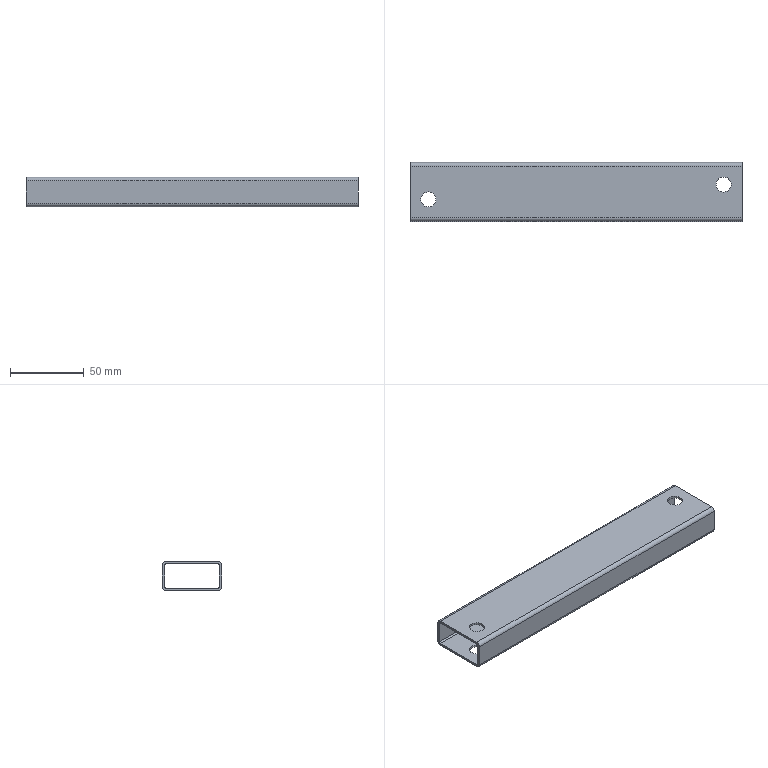Part | STEP file | 6150402 | 1 solid | 22 faces | box 225 x 40 x 20 mm | volume 36971 mm3 | cylinder 12 | plane 10 | commonest cylinder face diameters 2 x4 5 x4 10.2 x4
STEP:
#1=CARTESIAN_POINT('',(225.,17.5,-10.));
#2=VERTEX_POINT('',#1);
#3=CARTESIAN_POINT('',(225.,20.,-7.5));
#4=VERTEX_POINT('',#3);
#5=CARTESIAN_POINT('',(225.,17.5,-7.5));
#6=DIRECTION('',(1.,0.,0.));
#7=DIRECTION('',(0.,0.,-1.));
#8=AXIS2_PLACEMENT_3D('',#5,#6,#7);
#9=CIRCLE('',#8,2.5);
#10=EDGE_CURVE('',#2,#4,#9,.T.);
#11=ORIENTED_EDGE('',*,*,#10,.T.);
#12=CARTESIAN_POINT('',(225.,20.,7.5));
#13=VERTEX_POINT('',#12);
#14=CARTESIAN_POINT('',(225.,20.,7.5));
#15=DIRECTION('',(0.,0.,1.));
#16=VECTOR('',#15,1000.);
#17=LINE('',#14,#16);
#18=EDGE_CURVE('',#4,#13,#17,.T.);
#19=ORIENTED_EDGE('',*,*,#18,.T.);
#20=CARTESIAN_POINT('',(225.,17.5,10.));
#21=VERTEX_POINT('',#20);
#22=CARTESIAN_POINT('',(225.,17.5,7.5));
#23=DIRECTION('',(1.,0.,0.));
#24=DIRECTION('',(0.,0.,-1.));
#25=AXIS2_PLACEMENT_3D('',#22,#23,#24);
#26=CIRCLE('',#25,2.5);
#27=EDGE_CURVE('',#13,#21,#26,.T.);
#28=ORIENTED_EDGE('',*,*,#27,.T.);
#29=CARTESIAN_POINT('',(225.,-17.5,10.));
#30=VERTEX_POINT('',#29);
#31=CARTESIAN_POINT('',(225.,17.5,10.));
#32=DIRECTION('',(0.,-1.,0.));
#33=VECTOR('',#32,1000.);
#34=LINE('',#31,#33);
#35=EDGE_CURVE('',#21,#30,#34,.T.);
#36=ORIENTED_EDGE('',*,*,#35,.T.);
#37=CARTESIAN_POINT('',(225.,-20.,7.5));
#38=VERTEX_POINT('',#37);
#39=CARTESIAN_POINT('',(225.,-17.5,7.5));
#40=DIRECTION('',(1.,0.,0.));
#41=DIRECTION('',(0.,0.,-1.));
#42=AXIS2_PLACEMENT_3D('',#39,#40,#41);
#43=CIRCLE('',#42,2.5);
#44=EDGE_CURVE('',#30,#38,#43,.T.);
#45=ORIENTED_EDGE('',*,*,#44,.T.);
#46=CARTESIAN_POINT('',(225.,-20.,-7.5));
#47=VERTEX_POINT('',#46);
#48=CARTESIAN_POINT('',(225.,-20.,7.5));
#49=DIRECTION('',(0.,0.,-1.));
#50=VECTOR('',#49,1000.);
#51=LINE('',#48,#50);
#52=EDGE_CURVE('',#38,#47,#51,.T.);
#53=ORIENTED_EDGE('',*,*,#52,.T.);
#54=CARTESIAN_POINT('',(225.,-17.5,-10.));
#55=VERTEX_POINT('',#54);
#56=CARTESIAN_POINT('',(225.,-17.5,-7.5));
#57=DIRECTION('',(1.,0.,0.));
#58=DIRECTION('',(0.,0.,1.));
#59=AXIS2_PLACEMENT_3D('',#56,#57,#58);
#60=CIRCLE('',#59,2.5);
#61=EDGE_CURVE('',#47,#55,#60,.T.);
#62=ORIENTED_EDGE('',*,*,#61,.T.);
#63=CARTESIAN_POINT('',(225.,17.5,-10.));
#64=DIRECTION('',(0.,1.,0.));
#65=VECTOR('',#64,1000.);
#66=LINE('',#63,#65);
#67=EDGE_CURVE('',#55,#2,#66,.T.);
#68=ORIENTED_EDGE('',*,*,#67,.T.);
#69=EDGE_LOOP('',(#11,#19,#28,#36,#45,#53,#62,#68));
#70=FACE_OUTER_BOUND('',#69,.T.);
#71=CARTESIAN_POINT('',(225.,17.5,8.5));
#72=VERTEX_POINT('',#71);
#73=CARTESIAN_POINT('',(225.,-17.5,8.5));
#74=VERTEX_POINT('',#73);
#75=CARTESIAN_POINT('',(225.,17.5,8.5));
#76=DIRECTION('',(0.,-1.,0.));
#77=VECTOR('',#76,1000.);
#78=LINE('',#75,#77);
#79=EDGE_CURVE('',#72,#74,#78,.T.);
#80=ORIENTED_EDGE('',*,*,#79,.F.);
#81=CARTESIAN_POINT('',(225.,18.5,7.5));
#82=VERTEX_POINT('',#81);
#83=CARTESIAN_POINT('',(225.,17.5,7.5));
#84=DIRECTION('',(1.,0.,0.));
#85=DIRECTION('',(0.,0.,-1.));
#86=AXIS2_PLACEMENT_3D('',#83,#84,#85);
#87=CIRCLE('',#86,1.);
#88=EDGE_CURVE('',#82,#72,#87,.T.);
#89=ORIENTED_EDGE('',*,*,#88,.F.);
#90=CARTESIAN_POINT('',(225.,18.5,-7.5));
#91=VERTEX_POINT('',#90);
#92=CARTESIAN_POINT('',(225.,18.5,7.5));
#93=DIRECTION('',(0.,0.,1.));
#94=VECTOR('',#93,1000.);
#95=LINE('',#92,#94);
#96=EDGE_CURVE('',#91,#82,#95,.T.);
#97=ORIENTED_EDGE('',*,*,#96,.F.);
#98=CARTESIAN_POINT('',(225.,17.5,-8.5));
#99=VERTEX_POINT('',#98);
#100=CARTESIAN_POINT('',(225.,17.5,-7.5));
#101=DIRECTION('',(1.,0.,0.));
#102=DIRECTION('',(0.,0.,-1.));
#103=AXIS2_PLACEMENT_3D('',#100,#101,#102);
#104=CIRCLE('',#103,1.);
#105=EDGE_CURVE('',#99,#91,#104,.T.);
#106=ORIENTED_EDGE('',*,*,#105,.F.);
#107=CARTESIAN_POINT('',(225.,-17.5,-8.5));
#108=VERTEX_POINT('',#107);
#109=CARTESIAN_POINT('',(225.,17.5,-8.5));
#110=DIRECTION('',(0.,1.,0.));
#111=VECTOR('',#110,1000.);
#112=LINE('',#109,#111);
#113=EDGE_CURVE('',#108,#99,#112,.T.);
#114=ORIENTED_EDGE('',*,*,#113,.F.);
#115=CARTESIAN_POINT('',(225.,-18.5,-7.5));
#116=VERTEX_POINT('',#115);
#117=CARTESIAN_POINT('',(225.,-17.5,-7.5));
#118=DIRECTION('',(1.,0.,0.));
#119=DIRECTION('',(0.,0.,1.));
#120=AXIS2_PLACEMENT_3D('',#117,#118,#119);
#121=CIRCLE('',#120,1.);
#122=EDGE_CURVE('',#116,#108,#121,.T.);
#123=ORIENTED_EDGE('',*,*,#122,.F.);
#124=CARTESIAN_POINT('',(225.,-18.5,7.5));
#125=VERTEX_POINT('',#124);
#126=CARTESIAN_POINT('',(225.,-18.5,7.5));
#127=DIRECTION('',(0.,0.,-1.));
#128=VECTOR('',#127,1000.);
#129=LINE('',#126,#128);
#130=EDGE_CURVE('',#125,#116,#129,.T.);
#131=ORIENTED_EDGE('',*,*,#130,.F.);
#132=CARTESIAN_POINT('',(225.,-17.5,7.5));
#133=DIRECTION('',(1.,0.,0.));
#134=DIRECTION('',(0.,0.,-1.));
#135=AXIS2_PLACEMENT_3D('',#132,#133,#134);
#136=CIRCLE('',#135,1.);
#137=EDGE_CURVE('',#74,#125,#136,.T.);
#138=ORIENTED_EDGE('',*,*,#137,.F.);
#139=EDGE_LOOP('',(#80,#89,#97,#106,#114,#123,#131,#138));
#140=FACE_BOUND('',#139,.T.);
#141=CARTESIAN_POINT('',(225.,17.5,-7.5));
#142=DIRECTION('',(1.,0.,0.));
#143=DIRECTION('',(0.,0.,-1.));
#144=AXIS2_PLACEMENT_3D('',#141,#142,#143);
#145=PLANE('',#144);
#146=ADVANCED_FACE('',(#70,#140),#145,.T.);
#147=CARTESIAN_POINT('',(0.,17.5,-10.));
#148=VERTEX_POINT('',#147);
#149=CARTESIAN_POINT('',(0.,20.,-7.5));
#150=VERTEX_POINT('',#149);
#151=CARTESIAN_POINT('',(0.,17.5,-7.5));
#152=DIRECTION('',(1.,0.,0.));
#153=DIRECTION('',(0.,0.,-1.));
#154=AXIS2_PLACEMENT_3D('',#151,#152,#153);
#155=CIRCLE('',#154,2.5);
#156=EDGE_CURVE('',#148,#150,#155,.T.);
#157=ORIENTED_EDGE('',*,*,#156,.F.);
#158=CARTESIAN_POINT('',(0.,-17.5,-10.));
#159=VERTEX_POINT('',#158);
#160=CARTESIAN_POINT('',(0.,17.5,-10.));
#161=DIRECTION('',(0.,1.,0.));
#162=VECTOR('',#161,1000.);
#163=LINE('',#160,#162);
#164=EDGE_CURVE('',#159,#148,#163,.T.);
#165=ORIENTED_EDGE('',*,*,#164,.F.);
#166=CARTESIAN_POINT('',(0.,-20.,-7.5));
#167=VERTEX_POINT('',#166);
#168=CARTESIAN_POINT('',(0.,-17.5,-7.5));
#169=DIRECTION('',(1.,0.,0.));
#170=DIRECTION('',(0.,0.,1.));
#171=AXIS2_PLACEMENT_3D('',#168,#169,#170);
#172=CIRCLE('',#171,2.5);
#173=EDGE_CURVE('',#167,#159,#172,.T.);
#174=ORIENTED_EDGE('',*,*,#173,.F.);
#175=CARTESIAN_POINT('',(0.,-20.,7.5));
#176=VERTEX_POINT('',#175);
#177=CARTESIAN_POINT('',(0.,-20.,7.5));
#178=DIRECTION('',(0.,0.,-1.));
#179=VECTOR('',#178,1000.);
#180=LINE('',#177,#179);
#181=EDGE_CURVE('',#176,#167,#180,.T.);
#182=ORIENTED_EDGE('',*,*,#181,.F.);
#183=CARTESIAN_POINT('',(0.,-17.5,10.));
#184=VERTEX_POINT('',#183);
#185=CARTESIAN_POINT('',(0.,-17.5,7.5));
#186=DIRECTION('',(1.,0.,0.));
#187=DIRECTION('',(0.,0.,-1.));
#188=AXIS2_PLACEMENT_3D('',#185,#186,#187);
#189=CIRCLE('',#188,2.5);
#190=EDGE_CURVE('',#184,#176,#189,.T.);
#191=ORIENTED_EDGE('',*,*,#190,.F.);
#192=CARTESIAN_POINT('',(0.,17.5,10.));
#193=VERTEX_POINT('',#192);
#194=CARTESIAN_POINT('',(0.,17.5,10.));
#195=DIRECTION('',(0.,-1.,0.));
#196=VECTOR('',#195,1000.);
#197=LINE('',#194,#196);
#198=EDGE_CURVE('',#193,#184,#197,.T.);
#199=ORIENTED_EDGE('',*,*,#198,.F.);
#200=CARTESIAN_POINT('',(0.,20.,7.5));
#201=VERTEX_POINT('',#200);
#202=CARTESIAN_POINT('',(0.,17.5,7.5));
#203=DIRECTION('',(1.,0.,0.));
#204=DIRECTION('',(0.,0.,-1.));
#205=AXIS2_PLACEMENT_3D('',#202,#203,#204);
#206=CIRCLE('',#205,2.5);
#207=EDGE_CURVE('',#201,#193,#206,.T.);
#208=ORIENTED_EDGE('',*,*,#207,.F.);
#209=CARTESIAN_POINT('',(0.,20.,7.5));
#210=DIRECTION('',(0.,0.,1.));
#211=VECTOR('',#210,1000.);
#212=LINE('',#209,#211);
#213=EDGE_CURVE('',#150,#201,#212,.T.);
#214=ORIENTED_EDGE('',*,*,#213,.F.);
#215=EDGE_LOOP('',(#157,#165,#174,#182,#191,#199,#208,#214));
#216=FACE_OUTER_BOUND('',#215,.T.);
#217=CARTESIAN_POINT('',(0.,18.5,7.5));
#218=VERTEX_POINT('',#217);
#219=CARTESIAN_POINT('',(0.,17.5,8.5));
#220=VERTEX_POINT('',#219);
#221=CARTESIAN_POINT('',(0.,17.5,7.5));
#222=DIRECTION('',(1.,0.,0.));
#223=DIRECTION('',(0.,0.,-1.));
#224=AXIS2_PLACEMENT_3D('',#221,#222,#223);
#225=CIRCLE('',#224,1.);
#226=EDGE_CURVE('',#218,#220,#225,.T.);
#227=ORIENTED_EDGE('',*,*,#226,.T.);
#228=CARTESIAN_POINT('',(0.,-17.5,8.5));
#229=VERTEX_POINT('',#228);
#230=CARTESIAN_POINT('',(0.,17.5,8.5));
#231=DIRECTION('',(0.,-1.,0.));
#232=VECTOR('',#231,1000.);
#233=LINE('',#230,#232);
#234=EDGE_CURVE('',#220,#229,#233,.T.);
#235=ORIENTED_EDGE('',*,*,#234,.T.);
#236=CARTESIAN_POINT('',(0.,-18.5,7.5));
#237=VERTEX_POINT('',#236);
#238=CARTESIAN_POINT('',(0.,-17.5,7.5));
#239=DIRECTION('',(1.,0.,0.));
#240=DIRECTION('',(0.,0.,-1.));
#241=AXIS2_PLACEMENT_3D('',#238,#239,#240);
#242=CIRCLE('',#241,1.);
#243=EDGE_CURVE('',#229,#237,#242,.T.);
#244=ORIENTED_EDGE('',*,*,#243,.T.);
#245=CARTESIAN_POINT('',(0.,-18.5,-7.5));
#246=VERTEX_POINT('',#245);
#247=CARTESIAN_POINT('',(0.,-18.5,7.5));
#248=DIRECTION('',(0.,0.,-1.));
#249=VECTOR('',#248,1000.);
#250=LINE('',#247,#249);
#251=EDGE_CURVE('',#237,#246,#250,.T.);
#252=ORIENTED_EDGE('',*,*,#251,.T.);
#253=CARTESIAN_POINT('',(0.,-17.5,-8.5));
#254=VERTEX_POINT('',#253);
#255=CARTESIAN_POINT('',(0.,-17.5,-7.5));
#256=DIRECTION('',(1.,0.,0.));
#257=DIRECTION('',(0.,0.,1.));
#258=AXIS2_PLACEMENT_3D('',#255,#256,#257);
#259=CIRCLE('',#258,1.);
#260=EDGE_CURVE('',#246,#254,#259,.T.);
#261=ORIENTED_EDGE('',*,*,#260,.T.);
#262=CARTESIAN_POINT('',(0.,17.5,-8.5));
#263=VERTEX_POINT('',#262);
#264=CARTESIAN_POINT('',(0.,17.5,-8.5));
#265=DIRECTION('',(0.,1.,0.));
#266=VECTOR('',#265,1000.);
#267=LINE('',#264,#266);
#268=EDGE_CURVE('',#254,#263,#267,.T.);
#269=ORIENTED_EDGE('',*,*,#268,.T.);
#270=CARTESIAN_POINT('',(0.,18.5,-7.5));
#271=VERTEX_POINT('',#270);
#272=CARTESIAN_POINT('',(0.,17.5,-7.5));
#273=DIRECTION('',(1.,0.,0.));
#274=DIRECTION('',(0.,0.,-1.));
#275=AXIS2_PLACEMENT_3D('',#272,#273,#274);
#276=CIRCLE('',#275,1.);
#277=EDGE_CURVE('',#263,#271,#276,.T.);
#278=ORIENTED_EDGE('',*,*,#277,.T.);
#279=CARTESIAN_POINT('',(0.,18.5,7.5));
#280=DIRECTION('',(0.,0.,1.));
#281=VECTOR('',#280,1000.);
#282=LINE('',#279,#281);
#283=EDGE_CURVE('',#271,#218,#282,.T.);
#284=ORIENTED_EDGE('',*,*,#283,.T.);
#285=EDGE_LOOP('',(#227,#235,#244,#252,#261,#269,#278,#284));
#286=FACE_BOUND('',#285,.T.);
#287=CARTESIAN_POINT('',(0.,17.5,-7.5));
#288=DIRECTION('',(1.,0.,0.));
#289=DIRECTION('',(0.,0.,-1.));
#290=AXIS2_PLACEMENT_3D('',#287,#288,#289);
#291=PLANE('',#290);
#292=ADVANCED_FACE('',(#216,#286),#291,.F.);
#293=ORIENTED_EDGE('',*,*,#156,.T.);
#294=CARTESIAN_POINT('',(225.,20.,-7.5));
#295=DIRECTION('',(-1.,0.,0.));
#296=VECTOR('',#295,1000.);
#297=LINE('',#294,#296);
#298=EDGE_CURVE('',#4,#150,#297,.T.);
#299=ORIENTED_EDGE('',*,*,#298,.F.);
#300=ORIENTED_EDGE('',*,*,#10,.F.);
#301=CARTESIAN_POINT('',(225.,17.5,-10.));
#302=DIRECTION('',(-1.,0.,0.));
#303=VECTOR('',#302,1000.);
#304=LINE('',#301,#303);
#305=EDGE_CURVE('',#2,#148,#304,.T.);
#306=ORIENTED_EDGE('',*,*,#305,.T.);
#307=EDGE_LOOP('',(#293,#299,#300,#306));
#308=FACE_OUTER_BOUND('',#307,.T.);
#309=CARTESIAN_POINT('',(225.,17.5,-7.5));
#310=DIRECTION('',(-1.,0.,0.));
#311=DIRECTION('',(0.,0.,1.));
#312=AXIS2_PLACEMENT_3D('',#309,#310,#311);
#313=CYLINDRICAL_SURFACE('',#312,2.5);
#314=ADVANCED_FACE('',(#308),#313,.T.);
#315=ORIENTED_EDGE('',*,*,#213,.T.);
#316=CARTESIAN_POINT('',(225.,20.,7.5));
#317=DIRECTION('',(-1.,0.,0.));
#318=VECTOR('',#317,1000.);
#319=LINE('',#316,#318);
#320=EDGE_CURVE('',#13,#201,#319,.T.);
#321=ORIENTED_EDGE('',*,*,#320,.F.);
#322=ORIENTED_EDGE('',*,*,#18,.F.);
#323=ORIENTED_EDGE('',*,*,#298,.T.);
#324=EDGE_LOOP('',(#315,#321,#322,#323));
#325=FACE_OUTER_BOUND('',#324,.T.);
#326=CARTESIAN_POINT('',(225.,20.,7.5));
#327=DIRECTION('',(0.,-1.,0.));
#328=DIRECTION('',(0.,0.,-1.));
#329=AXIS2_PLACEMENT_3D('',#326,#327,#328);
#330=PLANE('',#329);
#331=ADVANCED_FACE('',(#325),#330,.F.);
#332=ORIENTED_EDGE('',*,*,#207,.T.);
#333=CARTESIAN_POINT('',(225.,17.5,10.));
#334=DIRECTION('',(-1.,0.,0.));
#335=VECTOR('',#334,1000.);
#336=LINE('',#333,#335);
#337=EDGE_CURVE('',#21,#193,#336,.T.);
#338=ORIENTED_EDGE('',*,*,#337,.F.);
#339=ORIENTED_EDGE('',*,*,#27,.F.);
#340=ORIENTED_EDGE('',*,*,#320,.T.);
#341=EDGE_LOOP('',(#332,#338,#339,#340));
#342=FACE_OUTER_BOUND('',#341,.T.);
#343=CARTESIAN_POINT('',(225.,17.5,7.5));
#344=DIRECTION('',(-1.,0.,0.));
#345=DIRECTION('',(0.,0.,1.));
#346=AXIS2_PLACEMENT_3D('',#343,#344,#345);
#347=CYLINDRICAL_SURFACE('',#346,2.5);
#348=ADVANCED_FACE('',(#342),#347,.T.);
#349=CARTESIAN_POINT('',(212.5,10.1,10.));
#350=VERTEX_POINT('',#349);
#351=CARTESIAN_POINT('',(212.5,5.,10.));
#352=DIRECTION('',(0.,0.,-1.));
#353=DIRECTION('',(0.,1.,0.));
#354=AXIS2_PLACEMENT_3D('',#351,#352,#353);
#355=CIRCLE('',#354,5.1);
#356=EDGE_CURVE('',#350,#350,#355,.T.);
#357=ORIENTED_EDGE('',*,*,#356,.T.);
#358=EDGE_LOOP('',(#357));
#359=FACE_BOUND('',#358,.T.);
#360=CARTESIAN_POINT('',(12.5,0.1,10.));
#361=VERTEX_POINT('',#360);
#362=CARTESIAN_POINT('',(12.5,-5.,10.));
#363=DIRECTION('',(0.,0.,-1.));
#364=DIRECTION('',(0.,1.,0.));
#365=AXIS2_PLACEMENT_3D('',#362,#363,#364);
#366=CIRCLE('',#365,5.1);
#367=EDGE_CURVE('',#361,#361,#366,.T.);
#368=ORIENTED_EDGE('',*,*,#367,.T.);
#369=EDGE_LOOP('',(#368));
#370=FACE_BOUND('',#369,.T.);
#371=ORIENTED_EDGE('',*,*,#198,.T.);
#372=CARTESIAN_POINT('',(225.,-17.5,10.));
#373=DIRECTION('',(-1.,0.,0.));
#374=VECTOR('',#373,1000.);
#375=LINE('',#372,#374);
#376=EDGE_CURVE('',#30,#184,#375,.T.);
#377=ORIENTED_EDGE('',*,*,#376,.F.);
#378=ORIENTED_EDGE('',*,*,#35,.F.);
#379=ORIENTED_EDGE('',*,*,#337,.T.);
#380=EDGE_LOOP('',(#371,#377,#378,#379));
#381=FACE_OUTER_BOUND('',#380,.T.);
#382=CARTESIAN_POINT('',(225.,17.5,10.));
#383=DIRECTION('',(0.,0.,-1.));
#384=DIRECTION('',(0.,1.,0.));
#385=AXIS2_PLACEMENT_3D('',#382,#383,#384);
#386=PLANE('',#385);
#387=ADVANCED_FACE('',(#359,#370,#381),#386,.F.);
#388=ORIENTED_EDGE('',*,*,#190,.T.);
#389=CARTESIAN_POINT('',(225.,-20.,7.5));
#390=DIRECTION('',(-1.,0.,0.));
#391=VECTOR('',#390,1000.);
#392=LINE('',#389,#391);
#393=EDGE_CURVE('',#38,#176,#392,.T.);
#394=ORIENTED_EDGE('',*,*,#393,.F.);
#395=ORIENTED_EDGE('',*,*,#44,.F.);
#396=ORIENTED_EDGE('',*,*,#376,.T.);
#397=EDGE_LOOP('',(#388,#394,#395,#396));
#398=FACE_OUTER_BOUND('',#397,.T.);
#399=CARTESIAN_POINT('',(225.,-17.5,7.5));
#400=DIRECTION('',(-1.,0.,0.));
#401=DIRECTION('',(0.,0.,1.));
#402=AXIS2_PLACEMENT_3D('',#399,#400,#401);
#403=CYLINDRICAL_SURFACE('',#402,2.5);
#404=ADVANCED_FACE('',(#398),#403,.T.);
#405=ORIENTED_EDGE('',*,*,#181,.T.);
#406=CARTESIAN_POINT('',(225.,-20.,-7.5));
#407=DIRECTION('',(-1.,0.,0.));
#408=VECTOR('',#407,1000.);
#409=LINE('',#406,#408);
#410=EDGE_CURVE('',#47,#167,#409,.T.);
#411=ORIENTED_EDGE('',*,*,#410,.F.);
#412=ORIENTED_EDGE('',*,*,#52,.F.);
#413=ORIENTED_EDGE('',*,*,#393,.T.);
#414=EDGE_LOOP('',(#405,#411,#412,#413));
#415=FACE_OUTER_BOUND('',#414,.T.);
#416=CARTESIAN_POINT('',(225.,-20.,7.5));
#417=DIRECTION('',(0.,1.,0.));
#418=DIRECTION('',(0.,0.,1.));
#419=AXIS2_PLACEMENT_3D('',#416,#417,#418);
#420=PLANE('',#419);
#421=ADVANCED_FACE('',(#415),#420,.F.);
#422=ORIENTED_EDGE('',*,*,#173,.T.);
#423=CARTESIAN_POINT('',(225.,-17.5,-10.));
#424=DIRECTION('',(-1.,0.,0.));
#425=VECTOR('',#424,1000.);
#426=LINE('',#423,#425);
#427=EDGE_CURVE('',#55,#159,#426,.T.);
#428=ORIENTED_EDGE('',*,*,#427,.F.);
#429=ORIENTED_EDGE('',*,*,#61,.F.);
#430=ORIENTED_EDGE('',*,*,#410,.T.);
#431=EDGE_LOOP('',(#422,#428,#429,#430));
#432=FACE_OUTER_BOUND('',#431,.T.);
#433=CARTESIAN_POINT('',(225.,-17.5,-7.5));
#434=DIRECTION('',(-1.,0.,0.));
#435=DIRECTION('',(0.,0.,1.));
#436=AXIS2_PLACEMENT_3D('',#433,#434,#435);
#437=CYLINDRICAL_SURFACE('',#436,2.5);
#438=ADVANCED_FACE('',(#432),#437,.T.);
#439=CARTESIAN_POINT('',(212.5,-0.1,-10.));
#440=VERTEX_POINT('',#439);
#441=CARTESIAN_POINT('',(212.5,5.,-10.));
#442=DIRECTION('',(0.,0.,1.));
#443=DIRECTION('',(0.,-1.,0.));
#444=AXIS2_PLACEMENT_3D('',#441,#442,#443);
#445=CIRCLE('',#444,5.1);
#446=EDGE_CURVE('',#440,#440,#445,.T.);
#447=ORIENTED_EDGE('',*,*,#446,.T.);
#448=EDGE_LOOP('',(#447));
#449=FACE_BOUND('',#448,.T.);
#450=CARTESIAN_POINT('',(12.5,-10.1,-10.));
#451=VERTEX_POINT('',#450);
#452=CARTESIAN_POINT('',(12.5,-5.,-10.));
#453=DIRECTION('',(0.,0.,1.));
#454=DIRECTION('',(0.,-1.,0.));
#455=AXIS2_PLACEMENT_3D('',#452,#453,#454);
#456=CIRCLE('',#455,5.1);
#457=EDGE_CURVE('',#451,#451,#456,.T.);
#458=ORIENTED_EDGE('',*,*,#457,.T.);
#459=EDGE_LOOP('',(#458));
#460=FACE_BOUND('',#459,.T.);
#461=ORIENTED_EDGE('',*,*,#164,.T.);
#462=ORIENTED_EDGE('',*,*,#305,.F.);
#463=ORIENTED_EDGE('',*,*,#67,.F.);
#464=ORIENTED_EDGE('',*,*,#427,.T.);
#465=EDGE_LOOP('',(#461,#462,#463,#464));
#466=FACE_OUTER_BOUND('',#465,.T.);
#467=CARTESIAN_POINT('',(225.,17.5,-10.));
#468=DIRECTION('',(0.,0.,1.));
#469=DIRECTION('',(0.,-1.,0.));
#470=AXIS2_PLACEMENT_3D('',#467,#468,#469);
#471=PLANE('',#470);
#472=ADVANCED_FACE('',(#449,#460,#466),#471,.F.);
#473=ORIENTED_EDGE('',*,*,#226,.F.);
#474=CARTESIAN_POINT('',(225.,18.5,7.5));
#475=DIRECTION('',(-1.,0.,0.));
#476=VECTOR('',#475,1000.);
#477=LINE('',#474,#476);
#478=EDGE_CURVE('',#82,#218,#477,.T.);
#479=ORIENTED_EDGE('',*,*,#478,.F.);
#480=ORIENTED_EDGE('',*,*,#88,.T.);
#481=CARTESIAN_POINT('',(225.,17.5,8.5));
#482=DIRECTION('',(-1.,0.,0.));
#483=VECTOR('',#482,1000.);
#484=LINE('',#481,#483);
#485=EDGE_CURVE('',#72,#220,#484,.T.);
#486=ORIENTED_EDGE('',*,*,#485,.T.);
#487=EDGE_LOOP('',(#473,#479,#480,#486));
#488=FACE_OUTER_BOUND('',#487,.T.);
#489=CARTESIAN_POINT('',(225.,17.5,7.5));
#490=DIRECTION('',(-1.,0.,0.));
#491=DIRECTION('',(0.,0.,1.));
#492=AXIS2_PLACEMENT_3D('',#489,#490,#491);
#493=CYLINDRICAL_SURFACE('',#492,1.);
#494=ADVANCED_FACE('',(#488),#493,.F.);
#495=CARTESIAN_POINT('',(212.5,10.1,8.5));
#496=VERTEX_POINT('',#495);
#497=CARTESIAN_POINT('',(212.5,5.,8.5));
#498=DIRECTION('',(0.,0.,-1.));
#499=DIRECTION('',(0.,1.,0.));
#500=AXIS2_PLACEMENT_3D('',#497,#498,#499);
#501=CIRCLE('',#500,5.1);
#502=EDGE_CURVE('',#496,#496,#501,.T.);
#503=ORIENTED_EDGE('',*,*,#502,.F.);
#504=EDGE_LOOP('',(#503));
#505=FACE_BOUND('',#504,.T.);
#506=CARTESIAN_POINT('',(12.5,0.1,8.5));
#507=VERTEX_POINT('',#506);
#508=CARTESIAN_POINT('',(12.5,-5.,8.5));
#509=DIRECTION('',(0.,0.,-1.));
#510=DIRECTION('',(0.,1.,0.));
#511=AXIS2_PLACEMENT_3D('',#508,#509,#510);
#512=CIRCLE('',#511,5.1);
#513=EDGE_CURVE('',#507,#507,#512,.T.);
#514=ORIENTED_EDGE('',*,*,#513,.F.);
#515=EDGE_LOOP('',(#514));
#516=FACE_BOUND('',#515,.T.);
#517=ORIENTED_EDGE('',*,*,#234,.F.);
#518=ORIENTED_EDGE('',*,*,#485,.F.);
#519=ORIENTED_EDGE('',*,*,#79,.T.);
#520=CARTESIAN_POINT('',(225.,-17.5,8.5));
#521=DIRECTION('',(-1.,0.,0.));
#522=VECTOR('',#521,1000.);
#523=LINE('',#520,#522);
#524=EDGE_CURVE('',#74,#229,#523,.T.);
#525=ORIENTED_EDGE('',*,*,#524,.T.);
#526=EDGE_LOOP('',(#517,#518,#519,#525));
#527=FACE_OUTER_BOUND('',#526,.T.);
#528=CARTESIAN_POINT('',(225.,17.5,8.5));
#529=DIRECTION('',(0.,0.,-1.));
#530=DIRECTION('',(0.,1.,0.));
#531=AXIS2_PLACEMENT_3D('',#528,#529,#530);
#532=PLANE('',#531);
#533=ADVANCED_FACE('',(#505,#516,#527),#532,.T.);
#534=ORIENTED_EDGE('',*,*,#243,.F.);
#535=ORIENTED_EDGE('',*,*,#524,.F.);
#536=ORIENTED_EDGE('',*,*,#137,.T.);
#537=CARTESIAN_POINT('',(225.,-18.5,7.5));
#538=DIRECTION('',(-1.,0.,0.));
#539=VECTOR('',#538,1000.);
#540=LINE('',#537,#539);
#541=EDGE_CURVE('',#125,#237,#540,.T.);
#542=ORIENTED_EDGE('',*,*,#541,.T.);
#543=EDGE_LOOP('',(#534,#535,#536,#542));
#544=FACE_OUTER_BOUND('',#543,.T.);
#545=CARTESIAN_POINT('',(225.,-17.5,7.5));
#546=DIRECTION('',(-1.,0.,0.));
#547=DIRECTION('',(0.,0.,1.));
#548=AXIS2_PLACEMENT_3D('',#545,#546,#547);
#549=CYLINDRICAL_SURFACE('',#548,1.);
#550=ADVANCED_FACE('',(#544),#549,.F.);
#551=ORIENTED_EDGE('',*,*,#251,.F.);
#552=ORIENTED_EDGE('',*,*,#541,.F.);
#553=ORIENTED_EDGE('',*,*,#130,.T.);
#554=CARTESIAN_POINT('',(225.,-18.5,-7.5));
#555=DIRECTION('',(-1.,0.,0.));
#556=VECTOR('',#555,1000.);
#557=LINE('',#554,#556);
#558=EDGE_CURVE('',#116,#246,#557,.T.);
#559=ORIENTED_EDGE('',*,*,#558,.T.);
#560=EDGE_LOOP('',(#551,#552,#553,#559));
#561=FACE_OUTER_BOUND('',#560,.T.);
#562=CARTESIAN_POINT('',(225.,-18.5,7.5));
#563=DIRECTION('',(0.,1.,0.));
#564=DIRECTION('',(0.,0.,1.));
#565=AXIS2_PLACEMENT_3D('',#562,#563,#564);
#566=PLANE('',#565);
#567=ADVANCED_FACE('',(#561),#566,.T.);
#568=ORIENTED_EDGE('',*,*,#260,.F.);
#569=ORIENTED_EDGE('',*,*,#558,.F.);
#570=ORIENTED_EDGE('',*,*,#122,.T.);
#571=CARTESIAN_POINT('',(225.,-17.5,-8.5));
#572=DIRECTION('',(-1.,0.,0.));
#573=VECTOR('',#572,1000.);
#574=LINE('',#571,#573);
#575=EDGE_CURVE('',#108,#254,#574,.T.);
#576=ORIENTED_EDGE('',*,*,#575,.T.);
#577=EDGE_LOOP('',(#568,#569,#570,#576));
#578=FACE_OUTER_BOUND('',#577,.T.);
#579=CARTESIAN_POINT('',(225.,-17.5,-7.5));
#580=DIRECTION('',(-1.,0.,0.));
#581=DIRECTION('',(0.,0.,1.));
#582=AXIS2_PLACEMENT_3D('',#579,#580,#581);
#583=CYLINDRICAL_SURFACE('',#582,1.);
#584=ADVANCED_FACE('',(#578),#583,.F.);
#585=CARTESIAN_POINT('',(212.5,-0.1,-8.5));
#586=VERTEX_POINT('',#585);
#587=CARTESIAN_POINT('',(212.5,5.,-8.5));
#588=DIRECTION('',(0.,0.,1.));
#589=DIRECTION('',(0.,-1.,0.));
#590=AXIS2_PLACEMENT_3D('',#587,#588,#589);
#591=CIRCLE('',#590,5.1);
#592=EDGE_CURVE('',#586,#586,#591,.T.);
#593=ORIENTED_EDGE('',*,*,#592,.F.);
#594=EDGE_LOOP('',(#593));
#595=FACE_BOUND('',#594,.T.);
#596=CARTESIAN_POINT('',(12.5,-10.1,-8.5));
#597=VERTEX_POINT('',#596);
#598=CARTESIAN_POINT('',(12.5,-5.,-8.5));
#599=DIRECTION('',(0.,0.,1.));
#600=DIRECTION('',(0.,-1.,0.));
#601=AXIS2_PLACEMENT_3D('',#598,#599,#600);
#602=CIRCLE('',#601,5.1);
#603=EDGE_CURVE('',#597,#597,#602,.T.);
#604=ORIENTED_EDGE('',*,*,#603,.F.);
#605=EDGE_LOOP('',(#604));
#606=FACE_BOUND('',#605,.T.);
#607=ORIENTED_EDGE('',*,*,#268,.F.);
#608=ORIENTED_EDGE('',*,*,#575,.F.);
#609=ORIENTED_EDGE('',*,*,#113,.T.);
#610=CARTESIAN_POINT('',(225.,17.5,-8.5));
#611=DIRECTION('',(-1.,0.,0.));
#612=VECTOR('',#611,1000.);
#613=LINE('',#610,#612);
#614=EDGE_CURVE('',#99,#263,#613,.T.);
#615=ORIENTED_EDGE('',*,*,#614,.T.);
#616=EDGE_LOOP('',(#607,#608,#609,#615));
#617=FACE_OUTER_BOUND('',#616,.T.);
#618=CARTESIAN_POINT('',(225.,17.5,-8.5));
#619=DIRECTION('',(0.,0.,1.));
#620=DIRECTION('',(0.,-1.,0.));
#621=AXIS2_PLACEMENT_3D('',#618,#619,#620);
#622=PLANE('',#621);
#623=ADVANCED_FACE('',(#595,#606,#617),#622,.T.);
#624=ORIENTED_EDGE('',*,*,#277,.F.);
#625=ORIENTED_EDGE('',*,*,#614,.F.);
#626=ORIENTED_EDGE('',*,*,#105,.T.);
#627=CARTESIAN_POINT('',(225.,18.5,-7.5));
#628=DIRECTION('',(-1.,0.,0.));
#629=VECTOR('',#628,1000.);
#630=LINE('',#627,#629);
#631=EDGE_CURVE('',#91,#271,#630,.T.);
#632=ORIENTED_EDGE('',*,*,#631,.T.);
#633=EDGE_LOOP('',(#624,#625,#626,#632));
#634=FACE_OUTER_BOUND('',#633,.T.);
#635=CARTESIAN_POINT('',(225.,17.5,-7.5));
#636=DIRECTION('',(-1.,0.,0.));
#637=DIRECTION('',(0.,0.,1.));
#638=AXIS2_PLACEMENT_3D('',#635,#636,#637);
#639=CYLINDRICAL_SURFACE('',#638,1.);
#640=ADVANCED_FACE('',(#634),#639,.F.);
#641=ORIENTED_EDGE('',*,*,#283,.F.);
#642=ORIENTED_EDGE('',*,*,#631,.F.);
#643=ORIENTED_EDGE('',*,*,#96,.T.);
#644=ORIENTED_EDGE('',*,*,#478,.T.);
#645=EDGE_LOOP('',(#641,#642,#643,#644));
#646=FACE_OUTER_BOUND('',#645,.T.);
#647=CARTESIAN_POINT('',(225.,18.5,7.5));
#648=DIRECTION('',(0.,-1.,0.));
#649=DIRECTION('',(0.,0.,-1.));
#650=AXIS2_PLACEMENT_3D('',#647,#648,#649);
#651=PLANE('',#650);
#652=ADVANCED_FACE('',(#646),#651,.T.);
#653=ORIENTED_EDGE('',*,*,#603,.T.);
#654=EDGE_LOOP('',(#653));
#655=FACE_OUTER_BOUND('',#654,.T.);
#656=ORIENTED_EDGE('',*,*,#457,.F.);
#657=EDGE_LOOP('',(#656));
#658=FACE_OUTER_BOUND('',#657,.T.);
#659=CARTESIAN_POINT('',(12.5,-5.,-15.));
#660=DIRECTION('',(0.,0.,1.));
#661=DIRECTION('',(1.,0.,0.));
#662=AXIS2_PLACEMENT_3D('',#659,#660,#661);
#663=CYLINDRICAL_SURFACE('',#662,5.1);
#664=ADVANCED_FACE('',(#655,#658),#663,.F.);
#665=ORIENTED_EDGE('',*,*,#513,.T.);
#666=EDGE_LOOP('',(#665));
#667=FACE_OUTER_BOUND('',#666,.T.);
#668=ORIENTED_EDGE('',*,*,#367,.F.);
#669=EDGE_LOOP('',(#668));
#670=FACE_OUTER_BOUND('',#669,.T.);
#671=CARTESIAN_POINT('',(12.5,-5.,-15.));
#672=DIRECTION('',(0.,0.,1.));
#673=DIRECTION('',(1.,0.,0.));
#674=AXIS2_PLACEMENT_3D('',#671,#672,#673);
#675=CYLINDRICAL_SURFACE('',#674,5.1);
#676=ADVANCED_FACE('',(#667,#670),#675,.F.);
#677=ORIENTED_EDGE('',*,*,#592,.T.);
#678=EDGE_LOOP('',(#677));
#679=FACE_OUTER_BOUND('',#678,.T.);
#680=ORIENTED_EDGE('',*,*,#446,.F.);
#681=EDGE_LOOP('',(#680));
#682=FACE_OUTER_BOUND('',#681,.T.);
#683=CARTESIAN_POINT('',(212.5,5.,-15.));
#684=DIRECTION('',(0.,0.,1.));
#685=DIRECTION('',(1.,0.,0.));
#686=AXIS2_PLACEMENT_3D('',#683,#684,#685);
#687=CYLINDRICAL_SURFACE('',#686,5.1);
#688=ADVANCED_FACE('',(#679,#682),#687,.F.);
#689=ORIENTED_EDGE('',*,*,#502,.T.);
#690=EDGE_LOOP('',(#689));
#691=FACE_OUTER_BOUND('',#690,.T.);
#692=ORIENTED_EDGE('',*,*,#356,.F.);
#693=EDGE_LOOP('',(#692));
#694=FACE_OUTER_BOUND('',#693,.T.);
#695=CARTESIAN_POINT('',(212.5,5.,-15.));
#696=DIRECTION('',(0.,0.,1.));
#697=DIRECTION('',(1.,0.,0.));
#698=AXIS2_PLACEMENT_3D('',#695,#696,#697);
#699=CYLINDRICAL_SURFACE('',#698,5.1);
#700=ADVANCED_FACE('',(#691,#694),#699,.F.);
#701=CLOSED_SHELL('',(#146,#292,#314,#331,#348,#387,#404,#421,#438,#472,#494,#533,#550,#567,#584,#623,#640,#652,#664,#676,#688,#700));
#702=MANIFOLD_SOLID_BREP('',#701);
#703=CARTESIAN_POINT('',(0.,0.,0.));
#704=DIRECTION('',(0.,0.,1.));
#705=DIRECTION('',(1.,0.,0.));
#706=AXIS2_PLACEMENT_3D('',#703,#704,#705);
#707=(LENGTH_UNIT()NAMED_UNIT(*)SI_UNIT(.MILLI.,.METRE.));
#708=UNCERTAINTY_MEASURE_WITH_UNIT(LENGTH_MEASURE(0.00001),#707,'','');
#709=(NAMED_UNIT(*)PLANE_ANGLE_UNIT()SI_UNIT($,.RADIAN.));
#710=(NAMED_UNIT(*)SI_UNIT($,.STERADIAN.)SOLID_ANGLE_UNIT());
#711=(GEOMETRIC_REPRESENTATION_CONTEXT(3)GLOBAL_UNCERTAINTY_ASSIGNED_CONTEXT((#708))GLOBAL_UNIT_ASSIGNED_CONTEXT((#707,#709,#710))REPRESENTATION_CONTEXT('',''));
#712=ADVANCED_BREP_SHAPE_REPRESENTATION('',(#702,#706),#711);